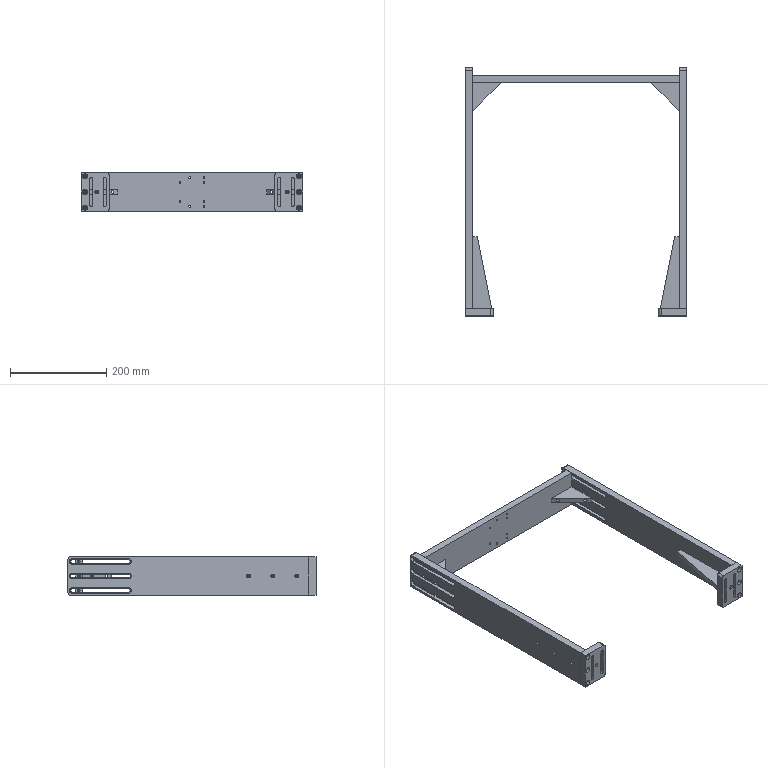Part | SolidWorks | 9 solids | 360 faces | box 460 x 515 x 80 mm | volume 1818663 mm3 | cylinder 200 | plane 120 | cone 40 | commonest cylinder face diameters 6.6 x44 11 x44 5 x40 3.3 x32 4.5 x16 8 x16